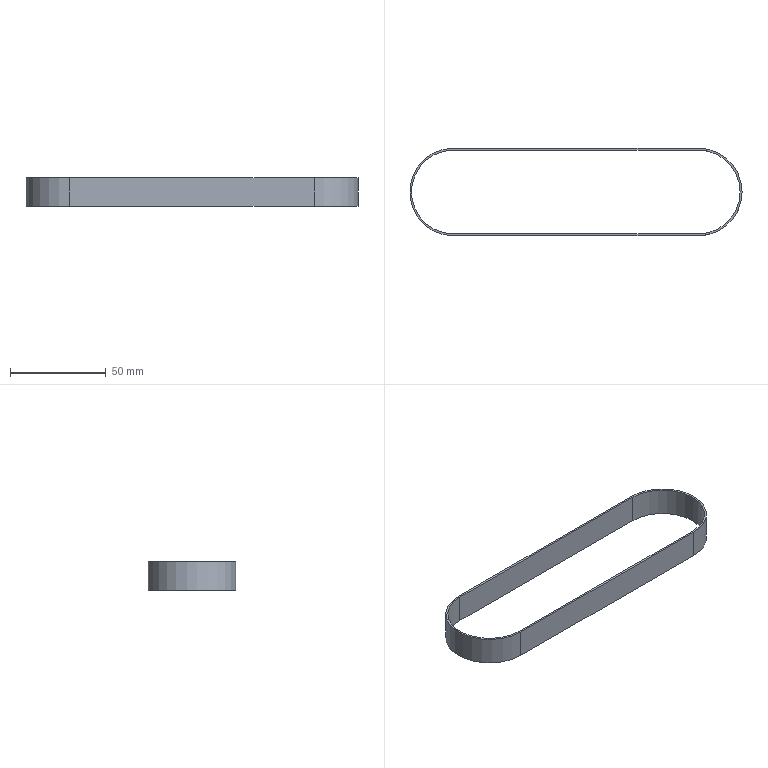Part | STEP file | 1 solid | 12 faces | box 173.39 x 45.75 x 15 mm | volume 5938 mm3 | cylinder 6 | plane 6 | commonest cylinder face diameters 43.75 x3 45.75 x3
STEP:
#1=CARTESIAN_POINT('',(0.,0.,0.));
#2=DIRECTION('',(0.,0.,1.));
#3=DIRECTION('',(1.,0.,0.));
#4=AXIS2_PLACEMENT_3D('',#1,#2,#3);
#5=CARTESIAN_POINT('',(63.82,-22.875,-7.5));
#6=VERTEX_POINT('',#5);
#7=CARTESIAN_POINT('',(86.695,0.,-7.5));
#8=VERTEX_POINT('',#7);
#9=CARTESIAN_POINT('',(63.82,0.,-7.5));
#10=DIRECTION('',(0.,0.,1.));
#11=DIRECTION('',(1.,0.,0.));
#12=AXIS2_PLACEMENT_3D('',#9,#10,#11);
#13=CIRCLE('',#12,22.875);
#14=CARTESIAN_POINT('',(63.82,0.,7.5));
#15=DIRECTION('',(0.,0.,1.));
#16=DIRECTION('',(1.,0.,0.));
#17=AXIS2_PLACEMENT_3D('',#14,#15,#16);
#18=CYLINDRICAL_SURFACE('',#17,22.875);
#19=CARTESIAN_POINT('',(0.,-15.));
#20=DIRECTION('',(1.,0.));
#21=VECTOR('',#20,1.);
#22=LINE('',#19,#21);
#23=(GEOMETRIC_REPRESENTATION_CONTEXT(2)PARAMETRIC_REPRESENTATION_CONTEXT()REPRESENTATION_CONTEXT('',''));
#24=DEFINITIONAL_REPRESENTATION('',(#22),#23);
#25=PCURVE('',#18,#24);
#26=CARTESIAN_POINT('',(-63.82,0.,-7.5));
#27=DIRECTION('',(0.,0.,1.));
#28=DIRECTION('',(1.,0.,0.));
#29=AXIS2_PLACEMENT_3D('',#26,#27,#28);
#30=PLANE('',#29);
#31=CARTESIAN_POINT('',(127.64,0.));
#32=DIRECTION('',(1.,0.));
#33=AXIS2_PLACEMENT_2D('',#31,#32);
#34=CIRCLE('',#33,22.875);
#35=(GEOMETRIC_REPRESENTATION_CONTEXT(2)PARAMETRIC_REPRESENTATION_CONTEXT()REPRESENTATION_CONTEXT('',''));
#36=DEFINITIONAL_REPRESENTATION('',(#34),#35);
#37=PCURVE('',#30,#36);
#38=SURFACE_CURVE('',#13,(#25,#37),.PCURVE_S1.);
#39=EDGE_CURVE('',#6,#8,#38,.T.);
#40=ORIENTED_EDGE('',*,*,#39,.T.);
#41=CARTESIAN_POINT('',(86.695,0.,7.5));
#42=VERTEX_POINT('',#41);
#43=CARTESIAN_POINT('',(86.695,0.,7.5));
#44=DIRECTION('',(0.,0.,1.));
#45=VECTOR('',#44,1.);
#46=LINE('',#43,#45);
#47=CARTESIAN_POINT('',(6.283,0.));
#48=DIRECTION('',(0.,1.));
#49=VECTOR('',#48,1.);
#50=LINE('',#47,#49);
#51=(GEOMETRIC_REPRESENTATION_CONTEXT(2)PARAMETRIC_REPRESENTATION_CONTEXT()REPRESENTATION_CONTEXT('',''));
#52=DEFINITIONAL_REPRESENTATION('',(#50),#51);
#53=PCURVE('',#18,#52);
#54=CARTESIAN_POINT('',(63.82,0.,7.5));
#55=DIRECTION('',(0.,0.,1.));
#56=DIRECTION('',(1.,0.,0.));
#57=AXIS2_PLACEMENT_3D('',#54,#55,#56);
#58=CYLINDRICAL_SURFACE('',#57,22.875);
#59=CARTESIAN_POINT('',(0.,0.));
#60=DIRECTION('',(0.,1.));
#61=VECTOR('',#60,1.);
#62=LINE('',#59,#61);
#63=(GEOMETRIC_REPRESENTATION_CONTEXT(2)PARAMETRIC_REPRESENTATION_CONTEXT()REPRESENTATION_CONTEXT('',''));
#64=DEFINITIONAL_REPRESENTATION('',(#62),#63);
#65=PCURVE('',#58,#64);
#66=SURFACE_CURVE('',#46,(#53,#65),.PCURVE_S1.);
#67=EDGE_CURVE('',#8,#42,#66,.T.);
#68=ORIENTED_EDGE('',*,*,#67,.T.);
#69=CARTESIAN_POINT('',(63.82,-22.875,7.5));
#70=VERTEX_POINT('',#69);
#71=CARTESIAN_POINT('',(63.82,0.,7.5));
#72=DIRECTION('',(0.,0.,-1.));
#73=DIRECTION('',(1.,0.,0.));
#74=AXIS2_PLACEMENT_3D('',#71,#72,#73);
#75=CIRCLE('',#74,22.875);
#76=CARTESIAN_POINT('',(6.283,0.));
#77=DIRECTION('',(-1.,0.));
#78=VECTOR('',#77,1.);
#79=LINE('',#76,#78);
#80=(GEOMETRIC_REPRESENTATION_CONTEXT(2)PARAMETRIC_REPRESENTATION_CONTEXT()REPRESENTATION_CONTEXT('',''));
#81=DEFINITIONAL_REPRESENTATION('',(#79),#80);
#82=PCURVE('',#18,#81);
#83=CARTESIAN_POINT('',(-63.82,0.,7.5));
#84=DIRECTION('',(0.,0.,1.));
#85=DIRECTION('',(1.,0.,0.));
#86=AXIS2_PLACEMENT_3D('',#83,#84,#85);
#87=PLANE('',#86);
#88=CARTESIAN_POINT('',(150.515,0.));
#89=CARTESIAN_POINT('',(150.515,-39.621));
#90=CARTESIAN_POINT('',(116.203,-19.81));
#91=CARTESIAN_POINT('',(81.89,0.));
#92=CARTESIAN_POINT('',(116.203,19.81));
#93=CARTESIAN_POINT('',(150.515,39.621));
#94=CARTESIAN_POINT('',(150.515,0.));
#95=(BOUNDED_CURVE()B_SPLINE_CURVE(2,(#88,#89,#90,#91,#92,#93,#94),.UNSPECIFIED.,.T.,.F.)B_SPLINE_CURVE_WITH_KNOTS((1,2,2,2,2,1),(-2.094,0.,2.094,4.189,6.283,8.378),.UNSPECIFIED.)CURVE()GEOMETRIC_REPRESENTATION_ITEM()RATIONAL_B_SPLINE_CURVE((1.,0.5,1.,0.5,1.,0.5,1.))REPRESENTATION_ITEM(''));
#96=(GEOMETRIC_REPRESENTATION_CONTEXT(2)PARAMETRIC_REPRESENTATION_CONTEXT()REPRESENTATION_CONTEXT('',''));
#97=DEFINITIONAL_REPRESENTATION('',(#95),#96);
#98=PCURVE('',#87,#97);
#99=SURFACE_CURVE('',#75,(#82,#98),.PCURVE_S1.);
#100=EDGE_CURVE('',#42,#70,#99,.T.);
#101=ORIENTED_EDGE('',*,*,#100,.T.);
#102=CARTESIAN_POINT('',(63.82,-22.875,7.5));
#103=DIRECTION('',(0.,0.,-1.));
#104=VECTOR('',#103,1.);
#105=LINE('',#102,#104);
#106=CARTESIAN_POINT('',(4.712,0.));
#107=DIRECTION('',(0.,-1.));
#108=VECTOR('',#107,1.);
#109=LINE('',#106,#108);
#110=(GEOMETRIC_REPRESENTATION_CONTEXT(2)PARAMETRIC_REPRESENTATION_CONTEXT()REPRESENTATION_CONTEXT('',''));
#111=DEFINITIONAL_REPRESENTATION('',(#109),#110);
#112=PCURVE('',#18,#111);
#113=CARTESIAN_POINT('',(-63.82,-22.875,7.5));
#114=DIRECTION('',(0.,1.,0.));
#115=DIRECTION('',(0.,0.,1.));
#116=AXIS2_PLACEMENT_3D('',#113,#114,#115);
#117=PLANE('',#116);
#118=CARTESIAN_POINT('',(0.,127.64));
#119=DIRECTION('',(-1.,0.));
#120=VECTOR('',#119,1.);
#121=LINE('',#118,#120);
#122=(GEOMETRIC_REPRESENTATION_CONTEXT(2)PARAMETRIC_REPRESENTATION_CONTEXT()REPRESENTATION_CONTEXT('',''));
#123=DEFINITIONAL_REPRESENTATION('',(#121),#122);
#124=PCURVE('',#117,#123);
#125=SURFACE_CURVE('',#105,(#112,#124),.PCURVE_S1.);
#126=EDGE_CURVE('',#70,#6,#125,.T.);
#127=ORIENTED_EDGE('',*,*,#126,.T.);
#128=EDGE_LOOP('',(#40,#68,#101,#127));
#129=FACE_BOUND('',#128,.T.);
#130=ADVANCED_FACE('',(#129),#18,.T.);
#131=CARTESIAN_POINT('',(63.82,21.875,-7.5));
#132=VERTEX_POINT('',#131);
#133=CARTESIAN_POINT('',(63.82,21.875,7.5));
#134=VERTEX_POINT('',#133);
#135=CARTESIAN_POINT('',(63.82,21.875,7.5));
#136=DIRECTION('',(0.,0.,1.));
#137=VECTOR('',#136,1.);
#138=LINE('',#135,#137);
#139=CARTESIAN_POINT('',(63.82,0.,7.5));
#140=DIRECTION('',(0.,0.,1.));
#141=DIRECTION('',(1.,0.,0.));
#142=AXIS2_PLACEMENT_3D('',#139,#140,#141);
#143=CYLINDRICAL_SURFACE('',#142,21.875);
#144=CARTESIAN_POINT('',(1.571,0.));
#145=DIRECTION('',(0.,1.));
#146=VECTOR('',#145,1.);
#147=LINE('',#144,#146);
#148=(GEOMETRIC_REPRESENTATION_CONTEXT(2)PARAMETRIC_REPRESENTATION_CONTEXT()REPRESENTATION_CONTEXT('',''));
#149=DEFINITIONAL_REPRESENTATION('',(#147),#148);
#150=PCURVE('',#143,#149);
#151=CARTESIAN_POINT('',(-63.82,21.875,7.5));
#152=DIRECTION('',(0.,-1.,0.));
#153=DIRECTION('',(1.,0.,0.));
#154=AXIS2_PLACEMENT_3D('',#151,#152,#153);
#155=PLANE('',#154);
#156=CARTESIAN_POINT('',(127.64,0.));
#157=DIRECTION('',(0.,1.));
#158=VECTOR('',#157,1.);
#159=LINE('',#156,#158);
#160=(GEOMETRIC_REPRESENTATION_CONTEXT(2)PARAMETRIC_REPRESENTATION_CONTEXT()REPRESENTATION_CONTEXT('',''));
#161=DEFINITIONAL_REPRESENTATION('',(#159),#160);
#162=PCURVE('',#155,#161);
#163=SURFACE_CURVE('',#138,(#150,#162),.PCURVE_S1.);
#164=EDGE_CURVE('',#132,#134,#163,.T.);
#165=ORIENTED_EDGE('',*,*,#164,.T.);
#166=CARTESIAN_POINT('',(85.695,0.,7.5));
#167=VERTEX_POINT('',#166);
#168=CARTESIAN_POINT('',(63.82,0.,7.5));
#169=DIRECTION('',(0.,0.,-1.));
#170=DIRECTION('',(1.,0.,0.));
#171=AXIS2_PLACEMENT_3D('',#168,#169,#170);
#172=CIRCLE('',#171,21.875);
#173=CARTESIAN_POINT('',(6.283,0.));
#174=DIRECTION('',(-1.,0.));
#175=VECTOR('',#174,1.);
#176=LINE('',#173,#175);
#177=(GEOMETRIC_REPRESENTATION_CONTEXT(2)PARAMETRIC_REPRESENTATION_CONTEXT()REPRESENTATION_CONTEXT('',''));
#178=DEFINITIONAL_REPRESENTATION('',(#176),#177);
#179=PCURVE('',#143,#178);
#180=CARTESIAN_POINT('',(149.515,0.));
#181=CARTESIAN_POINT('',(149.515,-37.889));
#182=CARTESIAN_POINT('',(116.703,-18.944));
#183=CARTESIAN_POINT('',(83.89,0.));
#184=CARTESIAN_POINT('',(116.703,18.944));
#185=CARTESIAN_POINT('',(149.515,37.889));
#186=CARTESIAN_POINT('',(149.515,0.));
#187=(BOUNDED_CURVE()B_SPLINE_CURVE(2,(#180,#181,#182,#183,#184,#185,#186),.UNSPECIFIED.,.T.,.F.)B_SPLINE_CURVE_WITH_KNOTS((1,2,2,2,2,1),(-2.094,0.,2.094,4.189,6.283,8.378),.UNSPECIFIED.)CURVE()GEOMETRIC_REPRESENTATION_ITEM()RATIONAL_B_SPLINE_CURVE((1.,0.5,1.,0.5,1.,0.5,1.))REPRESENTATION_ITEM(''));
#188=(GEOMETRIC_REPRESENTATION_CONTEXT(2)PARAMETRIC_REPRESENTATION_CONTEXT()REPRESENTATION_CONTEXT('',''));
#189=DEFINITIONAL_REPRESENTATION('',(#187),#188);
#190=PCURVE('',#87,#189);
#191=SURFACE_CURVE('',#172,(#179,#190),.PCURVE_S1.);
#192=EDGE_CURVE('',#134,#167,#191,.T.);
#193=ORIENTED_EDGE('',*,*,#192,.T.);
#194=CARTESIAN_POINT('',(85.695,0.,-7.5));
#195=VERTEX_POINT('',#194);
#196=CARTESIAN_POINT('',(85.695,0.,7.5));
#197=DIRECTION('',(0.,0.,1.));
#198=VECTOR('',#197,1.);
#199=LINE('',#196,#198);
#200=CARTESIAN_POINT('',(0.,0.));
#201=DIRECTION('',(0.,1.));
#202=VECTOR('',#201,1.);
#203=LINE('',#200,#202);
#204=(GEOMETRIC_REPRESENTATION_CONTEXT(2)PARAMETRIC_REPRESENTATION_CONTEXT()REPRESENTATION_CONTEXT('',''));
#205=DEFINITIONAL_REPRESENTATION('',(#203),#204);
#206=PCURVE('',#143,#205);
#207=CARTESIAN_POINT('',(63.82,0.,7.5));
#208=DIRECTION('',(0.,0.,1.));
#209=DIRECTION('',(1.,0.,0.));
#210=AXIS2_PLACEMENT_3D('',#207,#208,#209);
#211=CYLINDRICAL_SURFACE('',#210,21.875);
#212=CARTESIAN_POINT('',(6.283,0.));
#213=DIRECTION('',(0.,1.));
#214=VECTOR('',#213,1.);
#215=LINE('',#212,#214);
#216=(GEOMETRIC_REPRESENTATION_CONTEXT(2)PARAMETRIC_REPRESENTATION_CONTEXT()REPRESENTATION_CONTEXT('',''));
#217=DEFINITIONAL_REPRESENTATION('',(#215),#216);
#218=PCURVE('',#211,#217);
#219=SURFACE_CURVE('',#199,(#206,#218),.PCURVE_S1.);
#220=EDGE_CURVE('',#195,#167,#219,.T.);
#221=ORIENTED_EDGE('',*,*,#220,.F.);
#222=CARTESIAN_POINT('',(63.82,0.,-7.5));
#223=DIRECTION('',(0.,0.,-1.));
#224=DIRECTION('',(1.,0.,0.));
#225=AXIS2_PLACEMENT_3D('',#222,#223,#224);
#226=CIRCLE('',#225,21.875);
#227=CARTESIAN_POINT('',(6.283,-15.));
#228=DIRECTION('',(-1.,0.));
#229=VECTOR('',#228,1.);
#230=LINE('',#227,#229);
#231=(GEOMETRIC_REPRESENTATION_CONTEXT(2)PARAMETRIC_REPRESENTATION_CONTEXT()REPRESENTATION_CONTEXT('',''));
#232=DEFINITIONAL_REPRESENTATION('',(#230),#231);
#233=PCURVE('',#143,#232);
#234=CARTESIAN_POINT('',(149.515,0.));
#235=CARTESIAN_POINT('',(149.515,-37.889));
#236=CARTESIAN_POINT('',(116.703,-18.944));
#237=CARTESIAN_POINT('',(83.89,0.));
#238=CARTESIAN_POINT('',(116.703,18.944));
#239=CARTESIAN_POINT('',(149.515,37.889));
#240=CARTESIAN_POINT('',(149.515,0.));
#241=(BOUNDED_CURVE()B_SPLINE_CURVE(2,(#234,#235,#236,#237,#238,#239,#240),.UNSPECIFIED.,.T.,.F.)B_SPLINE_CURVE_WITH_KNOTS((1,2,2,2,2,1),(-2.094,0.,2.094,4.189,6.283,8.378),.UNSPECIFIED.)CURVE()GEOMETRIC_REPRESENTATION_ITEM()RATIONAL_B_SPLINE_CURVE((1.,0.5,1.,0.5,1.,0.5,1.))REPRESENTATION_ITEM(''));
#242=(GEOMETRIC_REPRESENTATION_CONTEXT(2)PARAMETRIC_REPRESENTATION_CONTEXT()REPRESENTATION_CONTEXT('',''));
#243=DEFINITIONAL_REPRESENTATION('',(#241),#242);
#244=PCURVE('',#30,#243);
#245=SURFACE_CURVE('',#226,(#233,#244),.PCURVE_S1.);
#246=EDGE_CURVE('',#132,#195,#245,.T.);
#247=ORIENTED_EDGE('',*,*,#246,.F.);
#248=EDGE_LOOP('',(#165,#193,#221,#247));
#249=FACE_BOUND('',#248,.F.);
#250=ADVANCED_FACE('',(#249),#143,.F.);
#251=ORIENTED_EDGE('',*,*,#126,.F.);
#252=CARTESIAN_POINT('',(-63.82,-22.875,7.5));
#253=VERTEX_POINT('',#252);
#254=CARTESIAN_POINT('',(-63.82,-22.875,7.5));
#255=DIRECTION('',(1.,0.,0.));
#256=VECTOR('',#255,1.);
#257=LINE('',#254,#256);
#258=CARTESIAN_POINT('',(0.,0.));
#259=DIRECTION('',(0.,1.));
#260=VECTOR('',#259,1.);
#261=LINE('',#258,#260);
#262=(GEOMETRIC_REPRESENTATION_CONTEXT(2)PARAMETRIC_REPRESENTATION_CONTEXT()REPRESENTATION_CONTEXT('',''));
#263=DEFINITIONAL_REPRESENTATION('',(#261),#262);
#264=PCURVE('',#117,#263);
#265=CARTESIAN_POINT('',(0.,-22.875));
#266=DIRECTION('',(1.,0.));
#267=VECTOR('',#266,1.);
#268=LINE('',#265,#267);
#269=(GEOMETRIC_REPRESENTATION_CONTEXT(2)PARAMETRIC_REPRESENTATION_CONTEXT()REPRESENTATION_CONTEXT('',''));
#270=DEFINITIONAL_REPRESENTATION('',(#268),#269);
#271=PCURVE('',#87,#270);
#272=SURFACE_CURVE('',#257,(#264,#271),.PCURVE_S1.);
#273=EDGE_CURVE('',#253,#70,#272,.T.);
#274=ORIENTED_EDGE('',*,*,#273,.F.);
#275=CARTESIAN_POINT('',(-63.82,-22.875,-7.5));
#276=VERTEX_POINT('',#275);
#277=CARTESIAN_POINT('',(-63.82,-22.875,7.5));
#278=DIRECTION('',(0.,0.,1.));
#279=VECTOR('',#278,1.);
#280=LINE('',#277,#279);
#281=CARTESIAN_POINT('',(0.,0.));
#282=DIRECTION('',(1.,0.));
#283=VECTOR('',#282,1.);
#284=LINE('',#281,#283);
#285=(GEOMETRIC_REPRESENTATION_CONTEXT(2)PARAMETRIC_REPRESENTATION_CONTEXT()REPRESENTATION_CONTEXT('',''));
#286=DEFINITIONAL_REPRESENTATION('',(#284),#285);
#287=PCURVE('',#117,#286);
#288=CARTESIAN_POINT('',(-63.82,0.,7.5));
#289=DIRECTION('',(0.,0.,1.));
#290=DIRECTION('',(1.,0.,0.));
#291=AXIS2_PLACEMENT_3D('',#288,#289,#290);
#292=CYLINDRICAL_SURFACE('',#291,22.875);
#293=CARTESIAN_POINT('',(4.712,0.));
#294=DIRECTION('',(0.,1.));
#295=VECTOR('',#294,1.);
#296=LINE('',#293,#295);
#297=(GEOMETRIC_REPRESENTATION_CONTEXT(2)PARAMETRIC_REPRESENTATION_CONTEXT()REPRESENTATION_CONTEXT('',''));
#298=DEFINITIONAL_REPRESENTATION('',(#296),#297);
#299=PCURVE('',#292,#298);
#300=SURFACE_CURVE('',#280,(#287,#299),.PCURVE_S1.);
#301=EDGE_CURVE('',#276,#253,#300,.T.);
#302=ORIENTED_EDGE('',*,*,#301,.F.);
#303=CARTESIAN_POINT('',(-63.82,-22.875,-7.5));
#304=DIRECTION('',(-1.,0.,0.));
#305=VECTOR('',#304,1.);
#306=LINE('',#303,#305);
#307=CARTESIAN_POINT('',(-15.,0.));
#308=DIRECTION('',(0.,-1.));
#309=VECTOR('',#308,1.);
#310=LINE('',#307,#309);
#311=(GEOMETRIC_REPRESENTATION_CONTEXT(2)PARAMETRIC_REPRESENTATION_CONTEXT()REPRESENTATION_CONTEXT('',''));
#312=DEFINITIONAL_REPRESENTATION('',(#310),#311);
#313=PCURVE('',#117,#312);
#314=CARTESIAN_POINT('',(0.,-22.875));
#315=DIRECTION('',(-1.,0.));
#316=VECTOR('',#315,1.);
#317=LINE('',#314,#316);
#318=(GEOMETRIC_REPRESENTATION_CONTEXT(2)PARAMETRIC_REPRESENTATION_CONTEXT()REPRESENTATION_CONTEXT('',''));
#319=DEFINITIONAL_REPRESENTATION('',(#317),#318);
#320=PCURVE('',#30,#319);
#321=SURFACE_CURVE('',#306,(#313,#320),.PCURVE_S1.);
#322=EDGE_CURVE('',#6,#276,#321,.T.);
#323=ORIENTED_EDGE('',*,*,#322,.F.);
#324=EDGE_LOOP('',(#251,#274,#302,#323));
#325=FACE_BOUND('',#324,.T.);
#326=ADVANCED_FACE('',(#325),#117,.F.);
#327=CARTESIAN_POINT('',(-63.82,-21.875,-7.5));
#328=VERTEX_POINT('',#327);
#329=CARTESIAN_POINT('',(-63.82,21.875,-7.5));
#330=VERTEX_POINT('',#329);
#331=CARTESIAN_POINT('',(-63.82,0.,-7.5));
#332=DIRECTION('',(0.,0.,-1.));
#333=DIRECTION('',(1.,0.,0.));
#334=AXIS2_PLACEMENT_3D('',#331,#332,#333);
#335=CIRCLE('',#334,21.875);
#336=CARTESIAN_POINT('',(21.875,0.));
#337=CARTESIAN_POINT('',(21.875,-37.889));
#338=CARTESIAN_POINT('',(-10.938,-18.944));
#339=CARTESIAN_POINT('',(-43.75,0.));
#340=CARTESIAN_POINT('',(-10.938,18.944));
#341=CARTESIAN_POINT('',(21.875,37.889));
#342=CARTESIAN_POINT('',(21.875,0.));
#343=(BOUNDED_CURVE()B_SPLINE_CURVE(2,(#336,#337,#338,#339,#340,#341,#342),.UNSPECIFIED.,.T.,.F.)B_SPLINE_CURVE_WITH_KNOTS((1,2,2,2,2,1),(-2.094,0.,2.094,4.189,6.283,8.378),.UNSPECIFIED.)CURVE()GEOMETRIC_REPRESENTATION_ITEM()RATIONAL_B_SPLINE_CURVE((1.,0.5,1.,0.5,1.,0.5,1.))REPRESENTATION_ITEM(''));
#344=(GEOMETRIC_REPRESENTATION_CONTEXT(2)PARAMETRIC_REPRESENTATION_CONTEXT()REPRESENTATION_CONTEXT('',''));
#345=DEFINITIONAL_REPRESENTATION('',(#343),#344);
#346=PCURVE('',#30,#345);
#347=CARTESIAN_POINT('',(-63.82,0.,7.5));
#348=DIRECTION('',(0.,0.,1.));
#349=DIRECTION('',(1.,0.,0.));
#350=AXIS2_PLACEMENT_3D('',#347,#348,#349);
#351=CYLINDRICAL_SURFACE('',#350,21.875);
#352=CARTESIAN_POINT('',(6.283,-15.));
#353=DIRECTION('',(-1.,0.));
#354=VECTOR('',#353,1.);
#355=LINE('',#352,#354);
#356=(GEOMETRIC_REPRESENTATION_CONTEXT(2)PARAMETRIC_REPRESENTATION_CONTEXT()REPRESENTATION_CONTEXT('',''));
#357=DEFINITIONAL_REPRESENTATION('',(#355),#356);
#358=PCURVE('',#351,#357);
#359=SURFACE_CURVE('',#335,(#346,#358),.PCURVE_S1.);
#360=EDGE_CURVE('',#328,#330,#359,.T.);
#361=ORIENTED_EDGE('',*,*,#360,.F.);
#362=CARTESIAN_POINT('',(63.82,-21.875,-7.5));
#363=VERTEX_POINT('',#362);
#364=CARTESIAN_POINT('',(-63.82,-21.875,-7.5));
#365=DIRECTION('',(-1.,0.,0.));
#366=VECTOR('',#365,1.);
#367=LINE('',#364,#366);
#368=CARTESIAN_POINT('',(0.,-21.875));
#369=DIRECTION('',(-1.,0.));
#370=VECTOR('',#369,1.);
#371=LINE('',#368,#370);
#372=(GEOMETRIC_REPRESENTATION_CONTEXT(2)PARAMETRIC_REPRESENTATION_CONTEXT()REPRESENTATION_CONTEXT('',''));
#373=DEFINITIONAL_REPRESENTATION('',(#371),#372);
#374=PCURVE('',#30,#373);
#375=CARTESIAN_POINT('',(-63.82,-21.875,7.5));
#376=DIRECTION('',(0.,1.,0.));
#377=DIRECTION('',(0.,0.,1.));
#378=AXIS2_PLACEMENT_3D('',#375,#376,#377);
#379=PLANE('',#378);
#380=CARTESIAN_POINT('',(-15.,0.));
#381=DIRECTION('',(0.,-1.));
#382=VECTOR('',#381,1.);
#383=LINE('',#380,#382);
#384=(GEOMETRIC_REPRESENTATION_CONTEXT(2)PARAMETRIC_REPRESENTATION_CONTEXT()REPRESENTATION_CONTEXT('',''));
#385=DEFINITIONAL_REPRESENTATION('',(#383),#384);
#386=PCURVE('',#379,#385);
#387=SURFACE_CURVE('',#367,(#374,#386),.PCURVE_S1.);
#388=EDGE_CURVE('',#363,#328,#387,.T.);
#389=ORIENTED_EDGE('',*,*,#388,.F.);
#390=CARTESIAN_POINT('',(63.82,0.,-7.5));
#391=DIRECTION('',(0.,0.,-1.));
#392=DIRECTION('',(1.,0.,0.));
#393=AXIS2_PLACEMENT_3D('',#390,#391,#392);
#394=CIRCLE('',#393,21.875);
#395=CARTESIAN_POINT('',(149.515,0.));
#396=CARTESIAN_POINT('',(149.515,-37.889));
#397=CARTESIAN_POINT('',(116.703,-18.944));
#398=CARTESIAN_POINT('',(83.89,0.));
#399=CARTESIAN_POINT('',(116.703,18.944));
#400=CARTESIAN_POINT('',(149.515,37.889));
#401=CARTESIAN_POINT('',(149.515,0.));
#402=(BOUNDED_CURVE()B_SPLINE_CURVE(2,(#395,#396,#397,#398,#399,#400,#401),.UNSPECIFIED.,.T.,.F.)B_SPLINE_CURVE_WITH_KNOTS((1,2,2,2,2,1),(-2.094,0.,2.094,4.189,6.283,8.378),.UNSPECIFIED.)CURVE()GEOMETRIC_REPRESENTATION_ITEM()RATIONAL_B_SPLINE_CURVE((1.,0.5,1.,0.5,1.,0.5,1.))REPRESENTATION_ITEM(''));
#403=(GEOMETRIC_REPRESENTATION_CONTEXT(2)PARAMETRIC_REPRESENTATION_CONTEXT()REPRESENTATION_CONTEXT('',''));
#404=DEFINITIONAL_REPRESENTATION('',(#402),#403);
#405=PCURVE('',#30,#404);
#406=CARTESIAN_POINT('',(6.283,-15.));
#407=DIRECTION('',(-1.,0.));
#408=VECTOR('',#407,1.);
#409=LINE('',#406,#408);
#410=(GEOMETRIC_REPRESENTATION_CONTEXT(2)PARAMETRIC_REPRESENTATION_CONTEXT()REPRESENTATION_CONTEXT('',''));
#411=DEFINITIONAL_REPRESENTATION('',(#409),#410);
#412=PCURVE('',#211,#411);
#413=SURFACE_CURVE('',#394,(#405,#412),.PCURVE_S1.);
#414=EDGE_CURVE('',#195,#363,#413,.T.);
#415=ORIENTED_EDGE('',*,*,#414,.F.);
#416=ORIENTED_EDGE('',*,*,#246,.F.);
#417=CARTESIAN_POINT('',(-63.82,21.875,-7.5));
#418=DIRECTION('',(1.,0.,0.));
#419=VECTOR('',#418,1.);
#420=LINE('',#417,#419);
#421=CARTESIAN_POINT('',(0.,21.875));
#422=DIRECTION('',(1.,0.));
#423=VECTOR('',#422,1.);
#424=LINE('',#421,#423);
#425=(GEOMETRIC_REPRESENTATION_CONTEXT(2)PARAMETRIC_REPRESENTATION_CONTEXT()REPRESENTATION_CONTEXT('',''));
#426=DEFINITIONAL_REPRESENTATION('',(#424),#425);
#427=PCURVE('',#30,#426);
#428=CARTESIAN_POINT('',(0.,-15.));
#429=DIRECTION('',(1.,0.));
#430=VECTOR('',#429,1.);
#431=LINE('',#428,#430);
#432=(GEOMETRIC_REPRESENTATION_CONTEXT(2)PARAMETRIC_REPRESENTATION_CONTEXT()REPRESENTATION_CONTEXT('',''));
#433=DEFINITIONAL_REPRESENTATION('',(#431),#432);
#434=PCURVE('',#155,#433);
#435=SURFACE_CURVE('',#420,(#427,#434),.PCURVE_S1.);
#436=EDGE_CURVE('',#330,#132,#435,.T.);
#437=ORIENTED_EDGE('',*,*,#436,.F.);
#438=EDGE_LOOP('',(#361,#389,#415,#416,#437));
#439=FACE_BOUND('',#438,.T.);
#440=CARTESIAN_POINT('',(63.82,22.875,-7.5));
#441=VERTEX_POINT('',#440);
#442=CARTESIAN_POINT('',(-63.82,22.875,-7.5));
#443=VERTEX_POINT('',#442);
#444=CARTESIAN_POINT('',(-63.82,22.875,-7.5));
#445=DIRECTION('',(-1.,0.,0.));
#446=VECTOR('',#445,1.);
#447=LINE('',#444,#446);
#448=CARTESIAN_POINT('',(0.,22.875));
#449=DIRECTION('',(-1.,0.));
#450=VECTOR('',#449,1.);
#451=LINE('',#448,#450);
#452=(GEOMETRIC_REPRESENTATION_CONTEXT(2)PARAMETRIC_REPRESENTATION_CONTEXT()REPRESENTATION_CONTEXT('',''));
#453=DEFINITIONAL_REPRESENTATION('',(#451),#452);
#454=PCURVE('',#30,#453);
#455=CARTESIAN_POINT('',(-63.82,22.875,7.5));
#456=DIRECTION('',(0.,-1.,0.));
#457=DIRECTION('',(1.,0.,0.));
#458=AXIS2_PLACEMENT_3D('',#455,#456,#457);
#459=PLANE('',#458);
#460=CARTESIAN_POINT('',(0.,-15.));
#461=DIRECTION('',(-1.,0.));
#462=VECTOR('',#461,1.);
#463=LINE('',#460,#462);
#464=(GEOMETRIC_REPRESENTATION_CONTEXT(2)PARAMETRIC_REPRESENTATION_CONTEXT()REPRESENTATION_CONTEXT('',''));
#465=DEFINITIONAL_REPRESENTATION('',(#463),#464);
#466=PCURVE('',#459,#465);
#467=SURFACE_CURVE('',#447,(#454,#466),.PCURVE_S1.);
#468=EDGE_CURVE('',#441,#443,#467,.T.);
#469=ORIENTED_EDGE('',*,*,#468,.F.);
#470=CARTESIAN_POINT('',(63.82,0.,-7.5));
#471=DIRECTION('',(0.,0.,1.));
#472=DIRECTION('',(1.,0.,0.));
#473=AXIS2_PLACEMENT_3D('',#470,#471,#472);
#474=CIRCLE('',#473,22.875);
#475=CARTESIAN_POINT('',(127.64,0.));
#476=DIRECTION('',(1.,0.));
#477=AXIS2_PLACEMENT_2D('',#475,#476);
#478=CIRCLE('',#477,22.875);
#479=(GEOMETRIC_REPRESENTATION_CONTEXT(2)PARAMETRIC_REPRESENTATION_CONTEXT()REPRESENTATION_CONTEXT('',''));
#480=DEFINITIONAL_REPRESENTATION('',(#478),#479);
#481=PCURVE('',#30,#480);
#482=CARTESIAN_POINT('',(0.,-15.));
#483=DIRECTION('',(1.,0.));
#484=VECTOR('',#483,1.);
#485=LINE('',#482,#484);
#486=(GEOMETRIC_REPRESENTATION_CONTEXT(2)PARAMETRIC_REPRESENTATION_CONTEXT()REPRESENTATION_CONTEXT('',''));
#487=DEFINITIONAL_REPRESENTATION('',(#485),#486);
#488=PCURVE('',#58,#487);
#489=SURFACE_CURVE('',#474,(#481,#488),.PCURVE_S1.);
#490=EDGE_CURVE('',#8,#441,#489,.T.);
#491=ORIENTED_EDGE('',*,*,#490,.F.);
#492=ORIENTED_EDGE('',*,*,#39,.F.);
#493=ORIENTED_EDGE('',*,*,#322,.T.);
#494=CARTESIAN_POINT('',(-63.82,0.,-7.5));
#495=DIRECTION('',(0.,0.,1.));
#496=DIRECTION('',(1.,0.,0.));
#497=AXIS2_PLACEMENT_3D('',#494,#495,#496);
#498=CIRCLE('',#497,22.875);
#499=CARTESIAN_POINT('',(0.,0.));
#500=DIRECTION('',(1.,0.));
#501=AXIS2_PLACEMENT_2D('',#499,#500);
#502=CIRCLE('',#501,22.875);
#503=(GEOMETRIC_REPRESENTATION_CONTEXT(2)PARAMETRIC_REPRESENTATION_CONTEXT()REPRESENTATION_CONTEXT('',''));
#504=DEFINITIONAL_REPRESENTATION('',(#502),#503);
#505=PCURVE('',#30,#504);
#506=CARTESIAN_POINT('',(0.,-15.));
#507=DIRECTION('',(1.,0.));
#508=VECTOR('',#507,1.);
#509=LINE('',#506,#508);
#510=(GEOMETRIC_REPRESENTATION_CONTEXT(2)PARAMETRIC_REPRESENTATION_CONTEXT()REPRESENTATION_CONTEXT('',''));
#511=DEFINITIONAL_REPRESENTATION('',(#509),#510);
#512=PCURVE('',#292,#511);
#513=SURFACE_CURVE('',#498,(#505,#512),.PCURVE_S1.);
#514=EDGE_CURVE('',#443,#276,#513,.T.);
#515=ORIENTED_EDGE('',*,*,#514,.F.);
#516=EDGE_LOOP('',(#469,#491,#492,#493,#515));
#517=FACE_BOUND('',#516,.T.);
#518=ADVANCED_FACE('',(#439,#517),#30,.F.);
#519=ORIENTED_EDGE('',*,*,#67,.F.);
#520=ORIENTED_EDGE('',*,*,#490,.T.);
#521=CARTESIAN_POINT('',(63.82,22.875,7.5));
#522=VERTEX_POINT('',#521);
#523=CARTESIAN_POINT('',(63.82,22.875,7.5));
#524=DIRECTION('',(0.,0.,1.));
#525=VECTOR('',#524,1.);
#526=LINE('',#523,#525);
#527=CARTESIAN_POINT('',(1.571,0.));
#528=DIRECTION('',(0.,1.));
#529=VECTOR('',#528,1.);
#530=LINE('',#527,#529);
#531=(GEOMETRIC_REPRESENTATION_CONTEXT(2)PARAMETRIC_REPRESENTATION_CONTEXT()REPRESENTATION_CONTEXT('',''));
#532=DEFINITIONAL_REPRESENTATION('',(#530),#531);
#533=PCURVE('',#58,#532);
#534=CARTESIAN_POINT('',(127.64,0.));
#535=DIRECTION('',(0.,1.));
#536=VECTOR('',#535,1.);
#537=LINE('',#534,#536);
#538=(GEOMETRIC_REPRESENTATION_CONTEXT(2)PARAMETRIC_REPRESENTATION_CONTEXT()REPRESENTATION_CONTEXT('',''));
#539=DEFINITIONAL_REPRESENTATION('',(#537),#538);
#540=PCURVE('',#459,#539);
#541=SURFACE_CURVE('',#526,(#533,#540),.PCURVE_S1.);
#542=EDGE_CURVE('',#441,#522,#541,.T.);
#543=ORIENTED_EDGE('',*,*,#542,.T.);
#544=CARTESIAN_POINT('',(63.82,0.,7.5));
#545=DIRECTION('',(0.,0.,-1.));
#546=DIRECTION('',(1.,0.,0.));
#547=AXIS2_PLACEMENT_3D('',#544,#545,#546);
#548=CIRCLE('',#547,22.875);
#549=CARTESIAN_POINT('',(6.283,0.));
#550=DIRECTION('',(-1.,0.));
#551=VECTOR('',#550,1.);
#552=LINE('',#549,#551);
#553=(GEOMETRIC_REPRESENTATION_CONTEXT(2)PARAMETRIC_REPRESENTATION_CONTEXT()REPRESENTATION_CONTEXT('',''));
#554=DEFINITIONAL_REPRESENTATION('',(#552),#553);
#555=PCURVE('',#58,#554);
#556=CARTESIAN_POINT('',(150.515,0.));
#557=CARTESIAN_POINT('',(150.515,-39.621));
#558=CARTESIAN_POINT('',(116.203,-19.81));
#559=CARTESIAN_POINT('',(81.89,0.));
#560=CARTESIAN_POINT('',(116.203,19.81));
#561=CARTESIAN_POINT('',(150.515,39.621));
#562=CARTESIAN_POINT('',(150.515,0.));
#563=(BOUNDED_CURVE()B_SPLINE_CURVE(2,(#556,#557,#558,#559,#560,#561,#562),.UNSPECIFIED.,.T.,.F.)B_SPLINE_CURVE_WITH_KNOTS((1,2,2,2,2,1),(-2.094,0.,2.094,4.189,6.283,8.378),.UNSPECIFIED.)CURVE()GEOMETRIC_REPRESENTATION_ITEM()RATIONAL_B_SPLINE_CURVE((1.,0.5,1.,0.5,1.,0.5,1.))REPRESENTATION_ITEM(''));
#564=(GEOMETRIC_REPRESENTATION_CONTEXT(2)PARAMETRIC_REPRESENTATION_CONTEXT()REPRESENTATION_CONTEXT('',''));
#565=DEFINITIONAL_REPRESENTATION('',(#563),#564);
#566=PCURVE('',#87,#565);
#567=SURFACE_CURVE('',#548,(#555,#566),.PCURVE_S1.);
#568=EDGE_CURVE('',#522,#42,#567,.T.);
#569=ORIENTED_EDGE('',*,*,#568,.T.);
#570=EDGE_LOOP('',(#519,#520,#543,#569));
#571=FACE_BOUND('',#570,.T.);
#572=ADVANCED_FACE('',(#571),#58,.T.);
#573=CARTESIAN_POINT('',(-63.82,21.875,7.5));
#574=VERTEX_POINT('',#573);
#575=CARTESIAN_POINT('',(-63.82,21.875,7.5));
#576=DIRECTION('',(1.,0.,0.));
#577=VECTOR('',#576,1.);
#578=LINE('',#575,#577);
#579=CARTESIAN_POINT('',(0.,21.875));
#580=DIRECTION('',(1.,0.));
#581=VECTOR('',#580,1.);
#582=LINE('',#579,#581);
#583=(GEOMETRIC_REPRESENTATION_CONTEXT(2)PARAMETRIC_REPRESENTATION_CONTEXT()REPRESENTATION_CONTEXT('',''));
#584=DEFINITIONAL_REPRESENTATION('',(#582),#583);
#585=PCURVE('',#87,#584);
#586=CARTESIAN_POINT('',(0.,0.));
#587=DIRECTION('',(1.,0.));
#588=VECTOR('',#587,1.);
#589=LINE('',#586,#588);
#590=(GEOMETRIC_REPRESENTATION_CONTEXT(2)PARAMETRIC_REPRESENTATION_CONTEXT()REPRESENTATION_CONTEXT('',''));
#591=DEFINITIONAL_REPRESENTATION('',(#589),#590);
#592=PCURVE('',#155,#591);
#593=SURFACE_CURVE('',#578,(#585,#592),.PCURVE_S1.);
#594=EDGE_CURVE('',#574,#134,#593,.T.);
#595=ORIENTED_EDGE('',*,*,#594,.T.);
#596=ORIENTED_EDGE('',*,*,#192,.T.);
#597=CARTESIAN_POINT('',(63.82,-21.875,7.5));
#598=VERTEX_POINT('',#597);
#599=CARTESIAN_POINT('',(63.82,0.,7.5));
#600=DIRECTION('',(0.,0.,-1.));
#601=DIRECTION('',(1.,0.,0.));
#602=AXIS2_PLACEMENT_3D('',#599,#600,#601);
#603=CIRCLE('',#602,21.875);
#604=CARTESIAN_POINT('',(149.515,0.));
#605=CARTESIAN_POINT('',(149.515,-37.889));
#606=CARTESIAN_POINT('',(116.703,-18.944));
#607=CARTESIAN_POINT('',(83.89,0.));
#608=CARTESIAN_POINT('',(116.703,18.944));
#609=CARTESIAN_POINT('',(149.515,37.889));
#610=CARTESIAN_POINT('',(149.515,0.));
#611=(BOUNDED_CURVE()B_SPLINE_CURVE(2,(#604,#605,#606,#607,#608,#609,#610),.UNSPECIFIED.,.T.,.F.)B_SPLINE_CURVE_WITH_KNOTS((1,2,2,2,2,1),(-2.094,0.,2.094,4.189,6.283,8.378),.UNSPECIFIED.)CURVE()GEOMETRIC_REPRESENTATION_ITEM()RATIONAL_B_SPLINE_CURVE((1.,0.5,1.,0.5,1.,0.5,1.))REPRESENTATION_ITEM(''));
#612=(GEOMETRIC_REPRESENTATION_CONTEXT(2)PARAMETRIC_REPRESENTATION_CONTEXT()REPRESENTATION_CONTEXT('',''));
#613=DEFINITIONAL_REPRESENTATION('',(#611),#612);
#614=PCURVE('',#87,#613);
#615=CARTESIAN_POINT('',(6.283,0.));
#616=DIRECTION('',(-1.,0.));
#617=VECTOR('',#616,1.);
#618=LINE('',#615,#617);
#619=(GEOMETRIC_REPRESENTATION_CONTEXT(2)PARAMETRIC_REPRESENTATION_CONTEXT()REPRESENTATION_CONTEXT('',''));
#620=DEFINITIONAL_REPRESENTATION('',(#618),#619);
#621=PCURVE('',#211,#620);
#622=SURFACE_CURVE('',#603,(#614,#621),.PCURVE_S1.);
#623=EDGE_CURVE('',#167,#598,#622,.T.);
#624=ORIENTED_EDGE('',*,*,#623,.T.);
#625=CARTESIAN_POINT('',(-63.82,-21.875,7.5));
#626=VERTEX_POINT('',#625);
#627=CARTESIAN_POINT('',(-63.82,-21.875,7.5));
#628=DIRECTION('',(-1.,0.,0.));
#629=VECTOR('',#628,1.);
#630=LINE('',#627,#629);
#631=CARTESIAN_POINT('',(0.,-21.875));
#632=DIRECTION('',(-1.,0.));
#633=VECTOR('',#632,1.);
#634=LINE('',#631,#633);
#635=(GEOMETRIC_REPRESENTATION_CONTEXT(2)PARAMETRIC_REPRESENTATION_CONTEXT()REPRESENTATION_CONTEXT('',''));
#636=DEFINITIONAL_REPRESENTATION('',(#634),#635);
#637=PCURVE('',#87,#636);
#638=CARTESIAN_POINT('',(0.,0.));
#639=DIRECTION('',(0.,-1.));
#640=VECTOR('',#639,1.);
#641=LINE('',#638,#640);
#642=(GEOMETRIC_REPRESENTATION_CONTEXT(2)PARAMETRIC_REPRESENTATION_CONTEXT()REPRESENTATION_CONTEXT('',''));
#643=DEFINITIONAL_REPRESENTATION('',(#641),#642);
#644=PCURVE('',#379,#643);
#645=SURFACE_CURVE('',#630,(#637,#644),.PCURVE_S1.);
#646=EDGE_CURVE('',#598,#626,#645,.T.);
#647=ORIENTED_EDGE('',*,*,#646,.T.);
#648=CARTESIAN_POINT('',(-63.82,0.,7.5));
#649=DIRECTION('',(0.,0.,-1.));
#650=DIRECTION('',(1.,0.,0.));
#651=AXIS2_PLACEMENT_3D('',#648,#649,#650);
#652=CIRCLE('',#651,21.875);
#653=CARTESIAN_POINT('',(21.875,0.));
#654=CARTESIAN_POINT('',(21.875,-37.889));
#655=CARTESIAN_POINT('',(-10.938,-18.944));
#656=CARTESIAN_POINT('',(-43.75,0.));
#657=CARTESIAN_POINT('',(-10.938,18.944));
#658=CARTESIAN_POINT('',(21.875,37.889));
#659=CARTESIAN_POINT('',(21.875,0.));
#660=(BOUNDED_CURVE()B_SPLINE_CURVE(2,(#653,#654,#655,#656,#657,#658,#659),.UNSPECIFIED.,.T.,.F.)B_SPLINE_CURVE_WITH_KNOTS((1,2,2,2,2,1),(-2.094,0.,2.094,4.189,6.283,8.378),.UNSPECIFIED.)CURVE()GEOMETRIC_REPRESENTATION_ITEM()RATIONAL_B_SPLINE_CURVE((1.,0.5,1.,0.5,1.,0.5,1.))REPRESENTATION_ITEM(''));
#661=(GEOMETRIC_REPRESENTATION_CONTEXT(2)PARAMETRIC_REPRESENTATION_CONTEXT()REPRESENTATION_CONTEXT('',''));
#662=DEFINITIONAL_REPRESENTATION('',(#660),#661);
#663=PCURVE('',#87,#662);
#664=CARTESIAN_POINT('',(6.283,0.));
#665=DIRECTION('',(-1.,0.));
#666=VECTOR('',#665,1.);
#667=LINE('',#664,#666);
#668=(GEOMETRIC_REPRESENTATION_CONTEXT(2)PARAMETRIC_REPRESENTATION_CONTEXT()REPRESENTATION_CONTEXT('',''));
#669=DEFINITIONAL_REPRESENTATION('',(#667),#668);
#670=PCURVE('',#351,#669);
#671=SURFACE_CURVE('',#652,(#663,#670),.PCURVE_S1.);
#672=EDGE_CURVE('',#626,#574,#671,.T.);
#673=ORIENTED_EDGE('',*,*,#672,.T.);
#674=EDGE_LOOP('',(#595,#596,#624,#647,#673));
#675=FACE_BOUND('',#674,.T.);
#676=ORIENTED_EDGE('',*,*,#568,.F.);
#677=CARTESIAN_POINT('',(-63.82,22.875,7.5));
#678=VERTEX_POINT('',#677);
#679=CARTESIAN_POINT('',(-63.82,22.875,7.5));
#680=DIRECTION('',(-1.,0.,0.));
#681=VECTOR('',#680,1.);
#682=LINE('',#679,#681);
#683=CARTESIAN_POINT('',(0.,22.875));
#684=DIRECTION('',(-1.,0.));
#685=VECTOR('',#684,1.);
#686=LINE('',#683,#685);
#687=(GEOMETRIC_REPRESENTATION_CONTEXT(2)PARAMETRIC_REPRESENTATION_CONTEXT()REPRESENTATION_CONTEXT('',''));
#688=DEFINITIONAL_REPRESENTATION('',(#686),#687);
#689=PCURVE('',#87,#688);
#690=CARTESIAN_POINT('',(0.,0.));
#691=DIRECTION('',(-1.,0.));
#692=VECTOR('',#691,1.);
#693=LINE('',#690,#692);
#694=(GEOMETRIC_REPRESENTATION_CONTEXT(2)PARAMETRIC_REPRESENTATION_CONTEXT()REPRESENTATION_CONTEXT('',''));
#695=DEFINITIONAL_REPRESENTATION('',(#693),#694);
#696=PCURVE('',#459,#695);
#697=SURFACE_CURVE('',#682,(#689,#696),.PCURVE_S1.);
#698=EDGE_CURVE('',#522,#678,#697,.T.);
#699=ORIENTED_EDGE('',*,*,#698,.T.);
#700=CARTESIAN_POINT('',(-63.82,0.,7.5));
#701=DIRECTION('',(0.,0.,1.));
#702=DIRECTION('',(1.,0.,0.));
#703=AXIS2_PLACEMENT_3D('',#700,#701,#702);
#704=CIRCLE('',#703,22.875);
#705=CARTESIAN_POINT('',(0.,0.));
#706=DIRECTION('',(1.,0.));
#707=AXIS2_PLACEMENT_2D('',#705,#706);
#708=CIRCLE('',#707,22.875);
#709=(GEOMETRIC_REPRESENTATION_CONTEXT(2)PARAMETRIC_REPRESENTATION_CONTEXT()REPRESENTATION_CONTEXT('',''));
#710=DEFINITIONAL_REPRESENTATION('',(#708),#709);
#711=PCURVE('',#87,#710);
#712=CARTESIAN_POINT('',(0.,0.));
#713=DIRECTION('',(1.,0.));
#714=VECTOR('',#713,1.);
#715=LINE('',#712,#714);
#716=(GEOMETRIC_REPRESENTATION_CONTEXT(2)PARAMETRIC_REPRESENTATION_CONTEXT()REPRESENTATION_CONTEXT('',''));
#717=DEFINITIONAL_REPRESENTATION('',(#715),#716);
#718=PCURVE('',#292,#717);
#719=SURFACE_CURVE('',#704,(#711,#718),.PCURVE_S1.);
#720=EDGE_CURVE('',#678,#253,#719,.T.);
#721=ORIENTED_EDGE('',*,*,#720,.T.);
#722=ORIENTED_EDGE('',*,*,#273,.T.);
#723=ORIENTED_EDGE('',*,*,#100,.F.);
#724=EDGE_LOOP('',(#676,#699,#721,#722,#723));
#725=FACE_BOUND('',#724,.T.);
#726=ADVANCED_FACE('',(#675,#725),#87,.T.);
#727=ORIENTED_EDGE('',*,*,#301,.T.);
#728=ORIENTED_EDGE('',*,*,#720,.F.);
#729=CARTESIAN_POINT('',(-63.82,22.875,7.5));
#730=DIRECTION('',(0.,0.,-1.));
#731=VECTOR('',#730,1.);
#732=LINE('',#729,#731);
#733=CARTESIAN_POINT('',(1.571,0.));
#734=DIRECTION('',(0.,-1.));
#735=VECTOR('',#734,1.);
#736=LINE('',#733,#735);
#737=(GEOMETRIC_REPRESENTATION_CONTEXT(2)PARAMETRIC_REPRESENTATION_CONTEXT()REPRESENTATION_CONTEXT('',''));
#738=DEFINITIONAL_REPRESENTATION('',(#736),#737);
#739=PCURVE('',#292,#738);
#740=CARTESIAN_POINT('',(0.,0.));
#741=DIRECTION('',(0.,-1.));
#742=VECTOR('',#741,1.);
#743=LINE('',#740,#742);
#744=(GEOMETRIC_REPRESENTATION_CONTEXT(2)PARAMETRIC_REPRESENTATION_CONTEXT()REPRESENTATION_CONTEXT('',''));
#745=DEFINITIONAL_REPRESENTATION('',(#743),#744);
#746=PCURVE('',#459,#745);
#747=SURFACE_CURVE('',#732,(#739,#746),.PCURVE_S1.);
#748=EDGE_CURVE('',#678,#443,#747,.T.);
#749=ORIENTED_EDGE('',*,*,#748,.T.);
#750=ORIENTED_EDGE('',*,*,#514,.T.);
#751=EDGE_LOOP('',(#727,#728,#749,#750));
#752=FACE_BOUND('',#751,.T.);
#753=ADVANCED_FACE('',(#752),#292,.T.);
#754=CARTESIAN_POINT('',(-63.82,-21.875,7.5));
#755=DIRECTION('',(0.,0.,1.));
#756=VECTOR('',#755,1.);
#757=LINE('',#754,#756);
#758=CARTESIAN_POINT('',(4.712,0.));
#759=DIRECTION('',(0.,1.));
#760=VECTOR('',#759,1.);
#761=LINE('',#758,#760);
#762=(GEOMETRIC_REPRESENTATION_CONTEXT(2)PARAMETRIC_REPRESENTATION_CONTEXT()REPRESENTATION_CONTEXT('',''));
#763=DEFINITIONAL_REPRESENTATION('',(#761),#762);
#764=PCURVE('',#351,#763);
#765=CARTESIAN_POINT('',(0.,0.));
#766=DIRECTION('',(1.,0.));
#767=VECTOR('',#766,1.);
#768=LINE('',#765,#767);
#769=(GEOMETRIC_REPRESENTATION_CONTEXT(2)PARAMETRIC_REPRESENTATION_CONTEXT()REPRESENTATION_CONTEXT('',''));
#770=DEFINITIONAL_REPRESENTATION('',(#768),#769);
#771=PCURVE('',#379,#770);
#772=SURFACE_CURVE('',#757,(#764,#771),.PCURVE_S1.);
#773=EDGE_CURVE('',#328,#626,#772,.T.);
#774=ORIENTED_EDGE('',*,*,#773,.T.);
#775=ORIENTED_EDGE('',*,*,#672,.T.);
#776=CARTESIAN_POINT('',(-63.82,21.875,7.5));
#777=DIRECTION('',(0.,0.,-1.));
#778=VECTOR('',#777,1.);
#779=LINE('',#776,#778);
#780=CARTESIAN_POINT('',(1.571,0.));
#781=DIRECTION('',(0.,-1.));
#782=VECTOR('',#781,1.);
#783=LINE('',#780,#782);
#784=(GEOMETRIC_REPRESENTATION_CONTEXT(2)PARAMETRIC_REPRESENTATION_CONTEXT()REPRESENTATION_CONTEXT('',''));
#785=DEFINITIONAL_REPRESENTATION('',(#783),#784);
#786=PCURVE('',#351,#785);
#787=CARTESIAN_POINT('',(0.,0.));
#788=DIRECTION('',(0.,-1.));
#789=VECTOR('',#788,1.);
#790=LINE('',#787,#789);
#791=(GEOMETRIC_REPRESENTATION_CONTEXT(2)PARAMETRIC_REPRESENTATION_CONTEXT()REPRESENTATION_CONTEXT('',''));
#792=DEFINITIONAL_REPRESENTATION('',(#790),#791);
#793=PCURVE('',#155,#792);
#794=SURFACE_CURVE('',#779,(#786,#793),.PCURVE_S1.);
#795=EDGE_CURVE('',#574,#330,#794,.T.);
#796=ORIENTED_EDGE('',*,*,#795,.T.);
#797=ORIENTED_EDGE('',*,*,#360,.F.);
#798=EDGE_LOOP('',(#774,#775,#796,#797));
#799=FACE_BOUND('',#798,.F.);
#800=ADVANCED_FACE('',(#799),#351,.F.);
#801=ORIENTED_EDGE('',*,*,#646,.F.);
#802=CARTESIAN_POINT('',(63.82,-21.875,7.5));
#803=DIRECTION('',(0.,0.,-1.));
#804=VECTOR('',#803,1.);
#805=LINE('',#802,#804);
#806=CARTESIAN_POINT('',(0.,127.64));
#807=DIRECTION('',(-1.,0.));
#808=VECTOR('',#807,1.);
#809=LINE('',#806,#808);
#810=(GEOMETRIC_REPRESENTATION_CONTEXT(2)PARAMETRIC_REPRESENTATION_CONTEXT()REPRESENTATION_CONTEXT('',''));
#811=DEFINITIONAL_REPRESENTATION('',(#809),#810);
#812=PCURVE('',#379,#811);
#813=CARTESIAN_POINT('',(4.712,0.));
#814=DIRECTION('',(0.,-1.));
#815=VECTOR('',#814,1.);
#816=LINE('',#813,#815);
#817=(GEOMETRIC_REPRESENTATION_CONTEXT(2)PARAMETRIC_REPRESENTATION_CONTEXT()REPRESENTATION_CONTEXT('',''));
#818=DEFINITIONAL_REPRESENTATION('',(#816),#817);
#819=PCURVE('',#211,#818);
#820=SURFACE_CURVE('',#805,(#812,#819),.PCURVE_S1.);
#821=EDGE_CURVE('',#598,#363,#820,.T.);
#822=ORIENTED_EDGE('',*,*,#821,.T.);
#823=ORIENTED_EDGE('',*,*,#388,.T.);
#824=ORIENTED_EDGE('',*,*,#773,.T.);
#825=EDGE_LOOP('',(#801,#822,#823,#824));
#826=FACE_BOUND('',#825,.T.);
#827=ADVANCED_FACE('',(#826),#379,.T.);
#828=ORIENTED_EDGE('',*,*,#623,.T.);
#829=ORIENTED_EDGE('',*,*,#821,.T.);
#830=ORIENTED_EDGE('',*,*,#414,.F.);
#831=ORIENTED_EDGE('',*,*,#220,.T.);
#832=EDGE_LOOP('',(#828,#829,#830,#831));
#833=FACE_BOUND('',#832,.F.);
#834=ADVANCED_FACE('',(#833),#211,.F.);
#835=ORIENTED_EDGE('',*,*,#594,.F.);
#836=ORIENTED_EDGE('',*,*,#795,.T.);
#837=ORIENTED_EDGE('',*,*,#436,.T.);
#838=ORIENTED_EDGE('',*,*,#164,.T.);
#839=EDGE_LOOP('',(#835,#836,#837,#838));
#840=FACE_BOUND('',#839,.T.);
#841=ADVANCED_FACE('',(#840),#155,.T.);
#842=ORIENTED_EDGE('',*,*,#748,.F.);
#843=ORIENTED_EDGE('',*,*,#698,.F.);
#844=ORIENTED_EDGE('',*,*,#542,.F.);
#845=ORIENTED_EDGE('',*,*,#468,.T.);
#846=EDGE_LOOP('',(#842,#843,#844,#845));
#847=FACE_BOUND('',#846,.T.);
#848=ADVANCED_FACE('',(#847),#459,.F.);
#849=CLOSED_SHELL('',(#130,#250,#326,#518,#572,#726,#753,#800,#827,#834,#841,#848));
#850=MANIFOLD_SOLID_BREP('',#849);
#851=(LENGTH_UNIT()NAMED_UNIT(*)SI_UNIT(.MILLI.,.METRE.));
#852=UNCERTAINTY_MEASURE_WITH_UNIT(LENGTH_MEASURE(0.0000001),#851,'','');
#853=(NAMED_UNIT(*)PLANE_ANGLE_UNIT()SI_UNIT($,.RADIAN.));
#854=(NAMED_UNIT(*)SI_UNIT($,.STERADIAN.)SOLID_ANGLE_UNIT());
#855=(GEOMETRIC_REPRESENTATION_CONTEXT(3)GLOBAL_UNCERTAINTY_ASSIGNED_CONTEXT((#852))GLOBAL_UNIT_ASSIGNED_CONTEXT((#851,#853,#854))REPRESENTATION_CONTEXT('',''));
#856=ADVANCED_BREP_SHAPE_REPRESENTATION('',(#4,#850),#855);